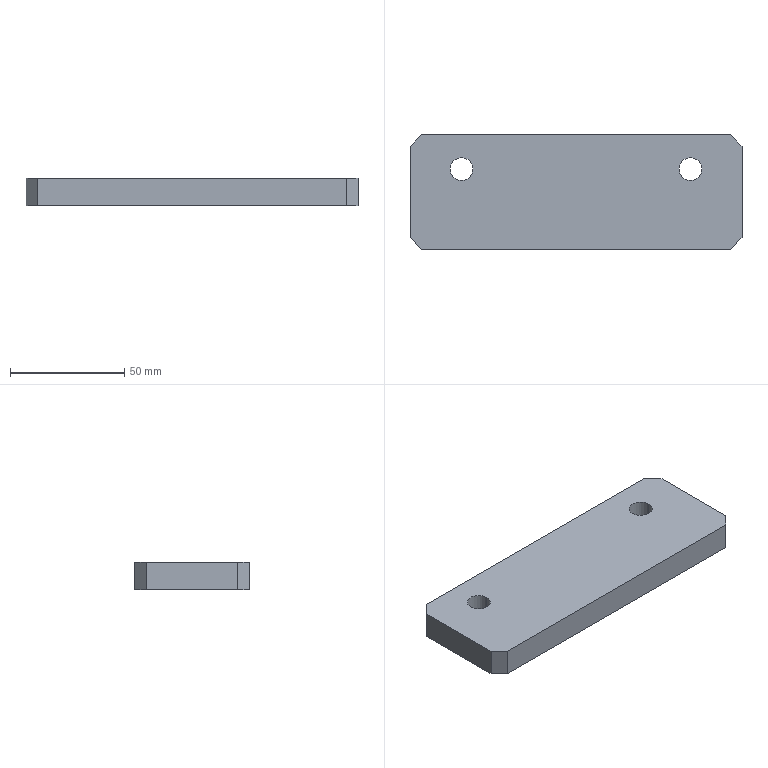Part | STEP file | [11] | 1 solid | 14 faces | box 145 x 50 x 12 mm | volume 84515 mm3 | plane 10 | cylinder 4 | commonest cylinder face diameters 10 x4
STEP:
#1=CARTESIAN_POINT('',(117.5,35.,-2.));
#2=VERTEX_POINT('',#1);
#3=CARTESIAN_POINT('',(127.5,35.,-2.));
#4=VERTEX_POINT('',#3);
#5=CARTESIAN_POINT('',(122.5,35.,-2.));
#6=DIRECTION('',(0.,0.,1.));
#7=DIRECTION('',(1.,0.,0.));
#8=AXIS2_PLACEMENT_3D('',#5,#6,#7);
#9=CIRCLE('',#8,5.);
#10=EDGE_CURVE('',#2,#4,#9,.T.);
#11=ORIENTED_EDGE('',*,*,#10,.F.);
#12=CARTESIAN_POINT('',(117.5,35.,10.));
#13=VERTEX_POINT('',#12);
#14=CARTESIAN_POINT('',(117.5,35.,-2.));
#15=DIRECTION('',(0.,0.,1.));
#16=VECTOR('',#15,1000.);
#17=LINE('',#14,#16);
#18=EDGE_CURVE('',#2,#13,#17,.T.);
#19=ORIENTED_EDGE('',*,*,#18,.T.);
#20=CARTESIAN_POINT('',(127.5,35.,10.));
#21=VERTEX_POINT('',#20);
#22=CARTESIAN_POINT('',(122.5,35.,10.));
#23=DIRECTION('',(0.,0.,-1.));
#24=DIRECTION('',(-1.,0.,0.));
#25=AXIS2_PLACEMENT_3D('',#22,#23,#24);
#26=CIRCLE('',#25,5.);
#27=EDGE_CURVE('',#21,#13,#26,.T.);
#28=ORIENTED_EDGE('',*,*,#27,.F.);
#29=CARTESIAN_POINT('',(127.5,35.,-2.));
#30=DIRECTION('',(0.,0.,1.));
#31=VECTOR('',#30,1000.);
#32=LINE('',#29,#31);
#33=EDGE_CURVE('',#4,#21,#32,.T.);
#34=ORIENTED_EDGE('',*,*,#33,.F.);
#35=EDGE_LOOP('',(#11,#19,#28,#34));
#36=FACE_OUTER_BOUND('',#35,.T.);
#37=CARTESIAN_POINT('',(122.5,35.,-2.));
#38=DIRECTION('',(0.,0.,1.));
#39=DIRECTION('',(1.,0.,0.));
#40=AXIS2_PLACEMENT_3D('',#37,#38,#39);
#41=CYLINDRICAL_SURFACE('',#40,5.);
#42=ADVANCED_FACE('',(#36),#41,.F.);
#43=CARTESIAN_POINT('',(17.5,35.,-2.));
#44=VERTEX_POINT('',#43);
#45=CARTESIAN_POINT('',(27.5,35.,-2.));
#46=VERTEX_POINT('',#45);
#47=CARTESIAN_POINT('',(22.5,35.,-2.));
#48=DIRECTION('',(0.,0.,1.));
#49=DIRECTION('',(1.,0.,0.));
#50=AXIS2_PLACEMENT_3D('',#47,#48,#49);
#51=CIRCLE('',#50,5.);
#52=EDGE_CURVE('',#44,#46,#51,.T.);
#53=ORIENTED_EDGE('',*,*,#52,.F.);
#54=CARTESIAN_POINT('',(17.5,35.,10.));
#55=VERTEX_POINT('',#54);
#56=CARTESIAN_POINT('',(17.5,35.,-2.));
#57=DIRECTION('',(0.,0.,1.));
#58=VECTOR('',#57,1000.);
#59=LINE('',#56,#58);
#60=EDGE_CURVE('',#44,#55,#59,.T.);
#61=ORIENTED_EDGE('',*,*,#60,.T.);
#62=CARTESIAN_POINT('',(27.5,35.,10.));
#63=VERTEX_POINT('',#62);
#64=CARTESIAN_POINT('',(22.5,35.,10.));
#65=DIRECTION('',(0.,0.,-1.));
#66=DIRECTION('',(-1.,0.,0.));
#67=AXIS2_PLACEMENT_3D('',#64,#65,#66);
#68=CIRCLE('',#67,5.);
#69=EDGE_CURVE('',#63,#55,#68,.T.);
#70=ORIENTED_EDGE('',*,*,#69,.F.);
#71=CARTESIAN_POINT('',(27.5,35.,-2.));
#72=DIRECTION('',(0.,0.,1.));
#73=VECTOR('',#72,1000.);
#74=LINE('',#71,#73);
#75=EDGE_CURVE('',#46,#63,#74,.T.);
#76=ORIENTED_EDGE('',*,*,#75,.F.);
#77=EDGE_LOOP('',(#53,#61,#70,#76));
#78=FACE_OUTER_BOUND('',#77,.T.);
#79=CARTESIAN_POINT('',(22.5,35.,-2.));
#80=DIRECTION('',(0.,0.,1.));
#81=DIRECTION('',(1.,0.,0.));
#82=AXIS2_PLACEMENT_3D('',#79,#80,#81);
#83=CYLINDRICAL_SURFACE('',#82,5.);
#84=ADVANCED_FACE('',(#78),#83,.F.);
#85=CARTESIAN_POINT('',(122.5,35.,-2.));
#86=DIRECTION('',(0.,0.,1.));
#87=DIRECTION('',(1.,0.,0.));
#88=AXIS2_PLACEMENT_3D('',#85,#86,#87);
#89=CIRCLE('',#88,5.);
#90=EDGE_CURVE('',#4,#2,#89,.T.);
#91=ORIENTED_EDGE('',*,*,#90,.T.);
#92=ORIENTED_EDGE('',*,*,#10,.T.);
#93=EDGE_LOOP('',(#91,#92));
#94=FACE_BOUND('',#93,.T.);
#95=CARTESIAN_POINT('',(22.5,35.,-2.));
#96=DIRECTION('',(0.,0.,1.));
#97=DIRECTION('',(1.,0.,0.));
#98=AXIS2_PLACEMENT_3D('',#95,#96,#97);
#99=CIRCLE('',#98,5.);
#100=EDGE_CURVE('',#46,#44,#99,.T.);
#101=ORIENTED_EDGE('',*,*,#100,.T.);
#102=ORIENTED_EDGE('',*,*,#52,.T.);
#103=EDGE_LOOP('',(#101,#102));
#104=FACE_BOUND('',#103,.T.);
#105=CARTESIAN_POINT('',(145.,5.,-2.));
#106=VERTEX_POINT('',#105);
#107=CARTESIAN_POINT('',(145.,45.,-2.));
#108=VERTEX_POINT('',#107);
#109=CARTESIAN_POINT('',(145.,25.,-2.));
#110=DIRECTION('',(0.,1.,0.));
#111=VECTOR('',#110,1000.);
#112=LINE('',#109,#111);
#113=EDGE_CURVE('',#106,#108,#112,.T.);
#114=ORIENTED_EDGE('',*,*,#113,.F.);
#115=CARTESIAN_POINT('',(140.,0.,-2.));
#116=VERTEX_POINT('',#115);
#117=CARTESIAN_POINT('',(118.75,-21.25,-2.));
#118=DIRECTION('',(-0.7071,-0.7071,0.));
#119=VECTOR('',#118,1000.);
#120=LINE('',#117,#119);
#121=EDGE_CURVE('',#106,#116,#120,.T.);
#122=ORIENTED_EDGE('',*,*,#121,.T.);
#123=CARTESIAN_POINT('',(5.,0.,-2.));
#124=VERTEX_POINT('',#123);
#125=CARTESIAN_POINT('',(72.5,0.,-2.));
#126=DIRECTION('',(1.,0.,0.));
#127=VECTOR('',#126,1000.);
#128=LINE('',#125,#127);
#129=EDGE_CURVE('',#124,#116,#128,.T.);
#130=ORIENTED_EDGE('',*,*,#129,.F.);
#131=CARTESIAN_POINT('',(0.,5.,-2.));
#132=VERTEX_POINT('',#131);
#133=CARTESIAN_POINT('',(26.25,-21.25,-2.));
#134=DIRECTION('',(-0.7071,0.7071,0.));
#135=VECTOR('',#134,1000.);
#136=LINE('',#133,#135);
#137=EDGE_CURVE('',#124,#132,#136,.T.);
#138=ORIENTED_EDGE('',*,*,#137,.T.);
#139=CARTESIAN_POINT('',(0.,45.,-2.));
#140=VERTEX_POINT('',#139);
#141=CARTESIAN_POINT('',(0.,25.,-2.));
#142=DIRECTION('',(0.,-1.,0.));
#143=VECTOR('',#142,1000.);
#144=LINE('',#141,#143);
#145=EDGE_CURVE('',#140,#132,#144,.T.);
#146=ORIENTED_EDGE('',*,*,#145,.F.);
#147=CARTESIAN_POINT('',(5.,50.,-2.));
#148=VERTEX_POINT('',#147);
#149=CARTESIAN_POINT('',(26.25,71.25,-2.));
#150=DIRECTION('',(0.7071,0.7071,0.));
#151=VECTOR('',#150,1000.);
#152=LINE('',#149,#151);
#153=EDGE_CURVE('',#140,#148,#152,.T.);
#154=ORIENTED_EDGE('',*,*,#153,.T.);
#155=CARTESIAN_POINT('',(140.,50.,-2.));
#156=VERTEX_POINT('',#155);
#157=CARTESIAN_POINT('',(72.5,50.,-2.));
#158=DIRECTION('',(-1.,0.,0.));
#159=VECTOR('',#158,1000.);
#160=LINE('',#157,#159);
#161=EDGE_CURVE('',#156,#148,#160,.T.);
#162=ORIENTED_EDGE('',*,*,#161,.F.);
#163=CARTESIAN_POINT('',(118.75,71.25,-2.));
#164=DIRECTION('',(0.7071,-0.7071,0.));
#165=VECTOR('',#164,1000.);
#166=LINE('',#163,#165);
#167=EDGE_CURVE('',#156,#108,#166,.T.);
#168=ORIENTED_EDGE('',*,*,#167,.T.);
#169=EDGE_LOOP('',(#114,#122,#130,#138,#146,#154,#162,#168));
#170=FACE_OUTER_BOUND('',#169,.T.);
#171=CARTESIAN_POINT('',(72.5,25.,-2.));
#172=DIRECTION('',(0.,0.,-1.));
#173=DIRECTION('',(-1.,0.,0.));
#174=AXIS2_PLACEMENT_3D('',#171,#172,#173);
#175=PLANE('',#174);
#176=ADVANCED_FACE('',(#94,#104,#170),#175,.T.);
#177=ORIENTED_EDGE('',*,*,#129,.T.);
#178=CARTESIAN_POINT('',(140.,0.,10.));
#179=VERTEX_POINT('',#178);
#180=CARTESIAN_POINT('',(140.,0.,10.));
#181=DIRECTION('',(0.,0.,1.));
#182=VECTOR('',#181,1000.);
#183=LINE('',#180,#182);
#184=EDGE_CURVE('',#116,#179,#183,.T.);
#185=ORIENTED_EDGE('',*,*,#184,.T.);
#186=CARTESIAN_POINT('',(5.,0.,10.));
#187=VERTEX_POINT('',#186);
#188=CARTESIAN_POINT('',(72.5,0.,10.));
#189=DIRECTION('',(-1.,0.,0.));
#190=VECTOR('',#189,1000.);
#191=LINE('',#188,#190);
#192=EDGE_CURVE('',#179,#187,#191,.T.);
#193=ORIENTED_EDGE('',*,*,#192,.T.);
#194=CARTESIAN_POINT('',(5.,0.,10.));
#195=DIRECTION('',(0.,0.,-1.));
#196=VECTOR('',#195,1000.);
#197=LINE('',#194,#196);
#198=EDGE_CURVE('',#187,#124,#197,.T.);
#199=ORIENTED_EDGE('',*,*,#198,.T.);
#200=EDGE_LOOP('',(#177,#185,#193,#199));
#201=FACE_OUTER_BOUND('',#200,.T.);
#202=CARTESIAN_POINT('',(72.5,0.,10.));
#203=DIRECTION('',(0.,-1.,0.));
#204=DIRECTION('',(0.,0.,1.));
#205=AXIS2_PLACEMENT_3D('',#202,#203,#204);
#206=PLANE('',#205);
#207=ADVANCED_FACE('',(#201),#206,.T.);
#208=CARTESIAN_POINT('',(145.,45.,10.));
#209=VERTEX_POINT('',#208);
#210=CARTESIAN_POINT('',(145.,5.,10.));
#211=VERTEX_POINT('',#210);
#212=CARTESIAN_POINT('',(145.,25.,10.));
#213=DIRECTION('',(0.,-1.,0.));
#214=VECTOR('',#213,1000.);
#215=LINE('',#212,#214);
#216=EDGE_CURVE('',#209,#211,#215,.T.);
#217=ORIENTED_EDGE('',*,*,#216,.T.);
#218=CARTESIAN_POINT('',(145.,5.,10.));
#219=DIRECTION('',(0.,0.,-1.));
#220=VECTOR('',#219,1000.);
#221=LINE('',#218,#220);
#222=EDGE_CURVE('',#211,#106,#221,.T.);
#223=ORIENTED_EDGE('',*,*,#222,.T.);
#224=ORIENTED_EDGE('',*,*,#113,.T.);
#225=CARTESIAN_POINT('',(145.,45.,10.));
#226=DIRECTION('',(0.,0.,1.));
#227=VECTOR('',#226,1000.);
#228=LINE('',#225,#227);
#229=EDGE_CURVE('',#108,#209,#228,.T.);
#230=ORIENTED_EDGE('',*,*,#229,.T.);
#231=EDGE_LOOP('',(#217,#223,#224,#230));
#232=FACE_OUTER_BOUND('',#231,.T.);
#233=CARTESIAN_POINT('',(145.,25.,10.));
#234=DIRECTION('',(1.,0.,0.));
#235=DIRECTION('',(0.,0.,-1.));
#236=AXIS2_PLACEMENT_3D('',#233,#234,#235);
#237=PLANE('',#236);
#238=ADVANCED_FACE('',(#232),#237,.T.);
#239=CARTESIAN_POINT('',(5.,50.,10.));
#240=VERTEX_POINT('',#239);
#241=CARTESIAN_POINT('',(140.,50.,10.));
#242=VERTEX_POINT('',#241);
#243=CARTESIAN_POINT('',(72.5,50.,10.));
#244=DIRECTION('',(1.,0.,0.));
#245=VECTOR('',#244,1000.);
#246=LINE('',#243,#245);
#247=EDGE_CURVE('',#240,#242,#246,.T.);
#248=ORIENTED_EDGE('',*,*,#247,.T.);
#249=CARTESIAN_POINT('',(140.,50.,10.));
#250=DIRECTION('',(0.,0.,-1.));
#251=VECTOR('',#250,1000.);
#252=LINE('',#249,#251);
#253=EDGE_CURVE('',#242,#156,#252,.T.);
#254=ORIENTED_EDGE('',*,*,#253,.T.);
#255=ORIENTED_EDGE('',*,*,#161,.T.);
#256=CARTESIAN_POINT('',(5.,50.,10.));
#257=DIRECTION('',(0.,0.,1.));
#258=VECTOR('',#257,1000.);
#259=LINE('',#256,#258);
#260=EDGE_CURVE('',#148,#240,#259,.T.);
#261=ORIENTED_EDGE('',*,*,#260,.T.);
#262=EDGE_LOOP('',(#248,#254,#255,#261));
#263=FACE_OUTER_BOUND('',#262,.T.);
#264=CARTESIAN_POINT('',(72.5,50.,10.));
#265=DIRECTION('',(0.,1.,0.));
#266=DIRECTION('',(0.,0.,-1.));
#267=AXIS2_PLACEMENT_3D('',#264,#265,#266);
#268=PLANE('',#267);
#269=ADVANCED_FACE('',(#263),#268,.T.);
#270=ORIENTED_EDGE('',*,*,#27,.T.);
#271=CARTESIAN_POINT('',(122.5,35.,10.));
#272=DIRECTION('',(0.,0.,-1.));
#273=DIRECTION('',(-1.,0.,0.));
#274=AXIS2_PLACEMENT_3D('',#271,#272,#273);
#275=CIRCLE('',#274,5.);
#276=EDGE_CURVE('',#13,#21,#275,.T.);
#277=ORIENTED_EDGE('',*,*,#276,.T.);
#278=EDGE_LOOP('',(#270,#277));
#279=FACE_BOUND('',#278,.T.);
#280=ORIENTED_EDGE('',*,*,#69,.T.);
#281=CARTESIAN_POINT('',(22.5,35.,10.));
#282=DIRECTION('',(0.,0.,-1.));
#283=DIRECTION('',(-1.,0.,0.));
#284=AXIS2_PLACEMENT_3D('',#281,#282,#283);
#285=CIRCLE('',#284,5.);
#286=EDGE_CURVE('',#55,#63,#285,.T.);
#287=ORIENTED_EDGE('',*,*,#286,.T.);
#288=EDGE_LOOP('',(#280,#287));
#289=FACE_BOUND('',#288,.T.);
#290=ORIENTED_EDGE('',*,*,#192,.F.);
#291=CARTESIAN_POINT('',(118.75,-21.25,10.));
#292=DIRECTION('',(0.7071,0.7071,0.));
#293=VECTOR('',#292,1000.);
#294=LINE('',#291,#293);
#295=EDGE_CURVE('',#179,#211,#294,.T.);
#296=ORIENTED_EDGE('',*,*,#295,.T.);
#297=ORIENTED_EDGE('',*,*,#216,.F.);
#298=CARTESIAN_POINT('',(118.75,71.25,10.));
#299=DIRECTION('',(-0.7071,0.7071,0.));
#300=VECTOR('',#299,1000.);
#301=LINE('',#298,#300);
#302=EDGE_CURVE('',#209,#242,#301,.T.);
#303=ORIENTED_EDGE('',*,*,#302,.T.);
#304=ORIENTED_EDGE('',*,*,#247,.F.);
#305=CARTESIAN_POINT('',(0.,45.,10.));
#306=VERTEX_POINT('',#305);
#307=CARTESIAN_POINT('',(26.25,71.25,10.));
#308=DIRECTION('',(-0.7071,-0.7071,0.));
#309=VECTOR('',#308,1000.);
#310=LINE('',#307,#309);
#311=EDGE_CURVE('',#240,#306,#310,.T.);
#312=ORIENTED_EDGE('',*,*,#311,.T.);
#313=CARTESIAN_POINT('',(0.,5.,10.));
#314=VERTEX_POINT('',#313);
#315=CARTESIAN_POINT('',(0.,25.,10.));
#316=DIRECTION('',(0.,1.,0.));
#317=VECTOR('',#316,1000.);
#318=LINE('',#315,#317);
#319=EDGE_CURVE('',#314,#306,#318,.T.);
#320=ORIENTED_EDGE('',*,*,#319,.F.);
#321=CARTESIAN_POINT('',(26.25,-21.25,10.));
#322=DIRECTION('',(0.7071,-0.7071,0.));
#323=VECTOR('',#322,1000.);
#324=LINE('',#321,#323);
#325=EDGE_CURVE('',#314,#187,#324,.T.);
#326=ORIENTED_EDGE('',*,*,#325,.T.);
#327=EDGE_LOOP('',(#290,#296,#297,#303,#304,#312,#320,#326));
#328=FACE_OUTER_BOUND('',#327,.T.);
#329=CARTESIAN_POINT('',(72.5,25.,10.));
#330=DIRECTION('',(0.,0.,1.));
#331=DIRECTION('',(1.,0.,0.));
#332=AXIS2_PLACEMENT_3D('',#329,#330,#331);
#333=PLANE('',#332);
#334=ADVANCED_FACE('',(#279,#289,#328),#333,.T.);
#335=ORIENTED_EDGE('',*,*,#145,.T.);
#336=CARTESIAN_POINT('',(0.,5.,10.));
#337=DIRECTION('',(0.,0.,1.));
#338=VECTOR('',#337,1000.);
#339=LINE('',#336,#338);
#340=EDGE_CURVE('',#132,#314,#339,.T.);
#341=ORIENTED_EDGE('',*,*,#340,.T.);
#342=ORIENTED_EDGE('',*,*,#319,.T.);
#343=CARTESIAN_POINT('',(0.,45.,10.));
#344=DIRECTION('',(0.,0.,-1.));
#345=VECTOR('',#344,1000.);
#346=LINE('',#343,#345);
#347=EDGE_CURVE('',#306,#140,#346,.T.);
#348=ORIENTED_EDGE('',*,*,#347,.T.);
#349=EDGE_LOOP('',(#335,#341,#342,#348));
#350=FACE_OUTER_BOUND('',#349,.T.);
#351=CARTESIAN_POINT('',(0.,25.,10.));
#352=DIRECTION('',(-1.,0.,0.));
#353=DIRECTION('',(0.,0.,1.));
#354=AXIS2_PLACEMENT_3D('',#351,#352,#353);
#355=PLANE('',#354);
#356=ADVANCED_FACE('',(#350),#355,.T.);
#357=ORIENTED_EDGE('',*,*,#325,.F.);
#358=ORIENTED_EDGE('',*,*,#340,.F.);
#359=ORIENTED_EDGE('',*,*,#137,.F.);
#360=ORIENTED_EDGE('',*,*,#198,.F.);
#361=EDGE_LOOP('',(#357,#358,#359,#360));
#362=FACE_OUTER_BOUND('',#361,.T.);
#363=CARTESIAN_POINT('',(5.,0.,10.));
#364=DIRECTION('',(0.7071,0.7071,0.));
#365=DIRECTION('',(0.,0.,-1.));
#366=AXIS2_PLACEMENT_3D('',#363,#364,#365);
#367=PLANE('',#366);
#368=ADVANCED_FACE('',(#362),#367,.F.);
#369=ORIENTED_EDGE('',*,*,#311,.F.);
#370=ORIENTED_EDGE('',*,*,#260,.F.);
#371=ORIENTED_EDGE('',*,*,#153,.F.);
#372=ORIENTED_EDGE('',*,*,#347,.F.);
#373=EDGE_LOOP('',(#369,#370,#371,#372));
#374=FACE_OUTER_BOUND('',#373,.T.);
#375=CARTESIAN_POINT('',(0.,45.,10.));
#376=DIRECTION('',(0.7071,-0.7071,0.));
#377=DIRECTION('',(0.,0.,-1.));
#378=AXIS2_PLACEMENT_3D('',#375,#376,#377);
#379=PLANE('',#378);
#380=ADVANCED_FACE('',(#374),#379,.F.);
#381=ORIENTED_EDGE('',*,*,#295,.F.);
#382=ORIENTED_EDGE('',*,*,#184,.F.);
#383=ORIENTED_EDGE('',*,*,#121,.F.);
#384=ORIENTED_EDGE('',*,*,#222,.F.);
#385=EDGE_LOOP('',(#381,#382,#383,#384));
#386=FACE_OUTER_BOUND('',#385,.T.);
#387=CARTESIAN_POINT('',(145.,5.,10.));
#388=DIRECTION('',(-0.7071,0.7071,0.));
#389=DIRECTION('',(0.,0.,-1.));
#390=AXIS2_PLACEMENT_3D('',#387,#388,#389);
#391=PLANE('',#390);
#392=ADVANCED_FACE('',(#386),#391,.F.);
#393=ORIENTED_EDGE('',*,*,#302,.F.);
#394=ORIENTED_EDGE('',*,*,#229,.F.);
#395=ORIENTED_EDGE('',*,*,#167,.F.);
#396=ORIENTED_EDGE('',*,*,#253,.F.);
#397=EDGE_LOOP('',(#393,#394,#395,#396));
#398=FACE_OUTER_BOUND('',#397,.T.);
#399=CARTESIAN_POINT('',(140.,50.,10.));
#400=DIRECTION('',(-0.7071,-0.7071,0.));
#401=DIRECTION('',(0.,0.,-1.));
#402=AXIS2_PLACEMENT_3D('',#399,#400,#401);
#403=PLANE('',#402);
#404=ADVANCED_FACE('',(#398),#403,.F.);
#405=ORIENTED_EDGE('',*,*,#60,.F.);
#406=ORIENTED_EDGE('',*,*,#100,.F.);
#407=ORIENTED_EDGE('',*,*,#75,.T.);
#408=ORIENTED_EDGE('',*,*,#286,.F.);
#409=EDGE_LOOP('',(#405,#406,#407,#408));
#410=FACE_OUTER_BOUND('',#409,.T.);
#411=CARTESIAN_POINT('',(22.5,35.,-2.));
#412=DIRECTION('',(0.,0.,1.));
#413=DIRECTION('',(1.,0.,0.));
#414=AXIS2_PLACEMENT_3D('',#411,#412,#413);
#415=CYLINDRICAL_SURFACE('',#414,5.);
#416=ADVANCED_FACE('',(#410),#415,.F.);
#417=ORIENTED_EDGE('',*,*,#18,.F.);
#418=ORIENTED_EDGE('',*,*,#90,.F.);
#419=ORIENTED_EDGE('',*,*,#33,.T.);
#420=ORIENTED_EDGE('',*,*,#276,.F.);
#421=EDGE_LOOP('',(#417,#418,#419,#420));
#422=FACE_OUTER_BOUND('',#421,.T.);
#423=CARTESIAN_POINT('',(122.5,35.,-2.));
#424=DIRECTION('',(0.,0.,1.));
#425=DIRECTION('',(1.,0.,0.));
#426=AXIS2_PLACEMENT_3D('',#423,#424,#425);
#427=CYLINDRICAL_SURFACE('',#426,5.);
#428=ADVANCED_FACE('',(#422),#427,.F.);
#429=CLOSED_SHELL('',(#42,#84,#176,#207,#238,#269,#334,#356,#368,#380,#392,#404,#416,#428));
#430=MANIFOLD_SOLID_BREP('',#429);
#431=CARTESIAN_POINT('',(0.,0.,0.));
#432=DIRECTION('',(0.,0.,1.));
#433=DIRECTION('',(1.,0.,0.));
#434=AXIS2_PLACEMENT_3D('',#431,#432,#433);
#435=(LENGTH_UNIT()NAMED_UNIT(*)SI_UNIT(.MILLI.,.METRE.));
#436=UNCERTAINTY_MEASURE_WITH_UNIT(LENGTH_MEASURE(0.00001),#435,'','');
#437=(NAMED_UNIT(*)PLANE_ANGLE_UNIT()SI_UNIT($,.RADIAN.));
#438=(NAMED_UNIT(*)SI_UNIT($,.STERADIAN.)SOLID_ANGLE_UNIT());
#439=(GEOMETRIC_REPRESENTATION_CONTEXT(3)GLOBAL_UNCERTAINTY_ASSIGNED_CONTEXT((#436))GLOBAL_UNIT_ASSIGNED_CONTEXT((#435,#437,#438))REPRESENTATION_CONTEXT('',''));
#440=ADVANCED_BREP_SHAPE_REPRESENTATION('',(#430,#434),#439);